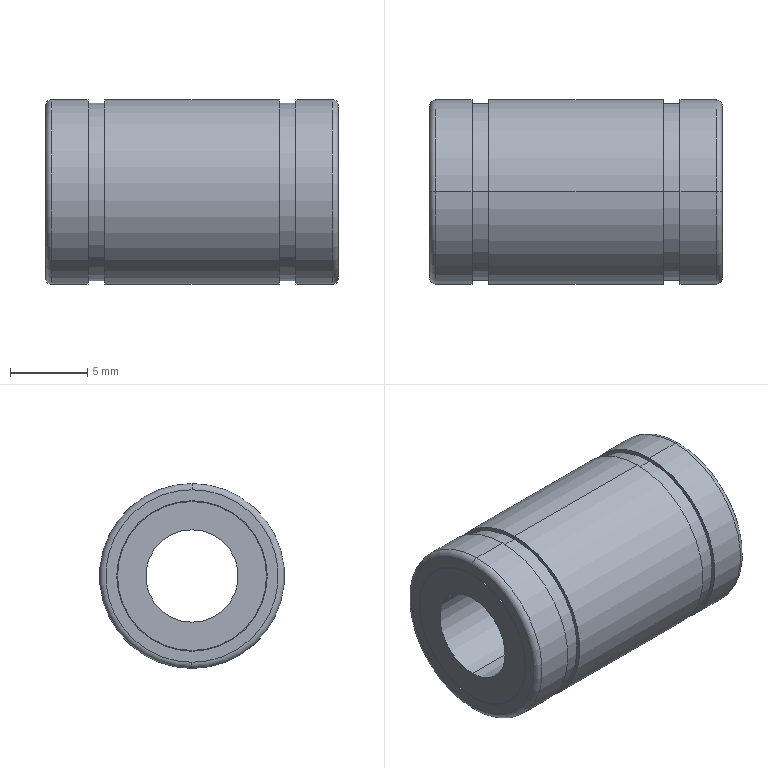Part | STEP file | 11-LMU6-A11_C-LMU6 | 1 solid | 34 faces | box 19 x 12 x 12 mm | volume 1589 mm3 | cylinder 20 | plane 10 | torus 4 | commonest cylinder face diameters 12 x6 9.667 x4 9.767 x4 11.5 x4 6 x2
STEP:
#1=CARTESIAN_POINT('',(9.5,0.,-3.));
#2=VERTEX_POINT('',#1);
#3=CARTESIAN_POINT('',(9.5,0.,3.));
#4=VERTEX_POINT('',#3);
#5=CARTESIAN_POINT('',(9.5,0.,0.));
#6=DIRECTION('',(-1.,0.,0.));
#7=DIRECTION('',(0.,0.,1.));
#8=AXIS2_PLACEMENT_3D('',#5,#6,#7);
#9=CIRCLE('',#8,3.);
#10=EDGE_CURVE('',#2,#4,#9,.T.);
#11=ORIENTED_EDGE('',*,*,#10,.F.);
#12=CARTESIAN_POINT('',(-9.5,0.,-3.));
#13=VERTEX_POINT('',#12);
#14=CARTESIAN_POINT('',(9.5,0.,-3.));
#15=DIRECTION('',(-1.,0.,0.));
#16=VECTOR('',#15,1000.);
#17=LINE('',#14,#16);
#18=EDGE_CURVE('',#2,#13,#17,.T.);
#19=ORIENTED_EDGE('',*,*,#18,.T.);
#20=CARTESIAN_POINT('',(-9.5,0.,3.));
#21=VERTEX_POINT('',#20);
#22=CARTESIAN_POINT('',(-9.5,0.,0.));
#23=DIRECTION('',(-1.,0.,0.));
#24=DIRECTION('',(0.,0.,1.));
#25=AXIS2_PLACEMENT_3D('',#22,#23,#24);
#26=CIRCLE('',#25,3.);
#27=EDGE_CURVE('',#13,#21,#26,.T.);
#28=ORIENTED_EDGE('',*,*,#27,.T.);
#29=CARTESIAN_POINT('',(9.5,0.,3.));
#30=DIRECTION('',(-1.,0.,0.));
#31=VECTOR('',#30,1000.);
#32=LINE('',#29,#31);
#33=EDGE_CURVE('',#4,#21,#32,.T.);
#34=ORIENTED_EDGE('',*,*,#33,.F.);
#35=EDGE_LOOP('',(#11,#19,#28,#34));
#36=FACE_OUTER_BOUND('',#35,.T.);
#37=CARTESIAN_POINT('',(9.5,0.,0.));
#38=DIRECTION('',(-1.,0.,0.));
#39=DIRECTION('',(0.,0.,1.));
#40=AXIS2_PLACEMENT_3D('',#37,#38,#39);
#41=CYLINDRICAL_SURFACE('',#40,3.);
#42=ADVANCED_FACE('',(#36),#41,.F.);
#43=CARTESIAN_POINT('',(9.5,0.,4.833));
#44=VERTEX_POINT('',#43);
#45=CARTESIAN_POINT('',(9.5,0.,-4.833));
#46=VERTEX_POINT('',#45);
#47=CARTESIAN_POINT('',(9.5,0.,0.));
#48=DIRECTION('',(-1.,0.,0.));
#49=DIRECTION('',(0.,0.,1.));
#50=AXIS2_PLACEMENT_3D('',#47,#48,#49);
#51=CIRCLE('',#50,4.833);
#52=EDGE_CURVE('',#44,#46,#51,.T.);
#53=ORIENTED_EDGE('',*,*,#52,.T.);
#54=CARTESIAN_POINT('',(9.45,0.,-4.833));
#55=VERTEX_POINT('',#54);
#56=CARTESIAN_POINT('',(9.5,0.,-4.833));
#57=DIRECTION('',(-1.,0.,0.));
#58=VECTOR('',#57,1000.);
#59=LINE('',#56,#58);
#60=EDGE_CURVE('',#46,#55,#59,.T.);
#61=ORIENTED_EDGE('',*,*,#60,.T.);
#62=CARTESIAN_POINT('',(9.45,0.,4.833));
#63=VERTEX_POINT('',#62);
#64=CARTESIAN_POINT('',(9.45,0.,0.));
#65=DIRECTION('',(1.,0.,0.));
#66=DIRECTION('',(0.,0.,1.));
#67=AXIS2_PLACEMENT_3D('',#64,#65,#66);
#68=CIRCLE('',#67,4.833);
#69=EDGE_CURVE('',#55,#63,#68,.T.);
#70=ORIENTED_EDGE('',*,*,#69,.T.);
#71=CARTESIAN_POINT('',(9.5,0.,4.833));
#72=DIRECTION('',(-1.,0.,0.));
#73=VECTOR('',#72,1000.);
#74=LINE('',#71,#73);
#75=EDGE_CURVE('',#44,#63,#74,.T.);
#76=ORIENTED_EDGE('',*,*,#75,.F.);
#77=EDGE_LOOP('',(#53,#61,#70,#76));
#78=FACE_OUTER_BOUND('',#77,.T.);
#79=CARTESIAN_POINT('',(9.5,0.,0.));
#80=DIRECTION('',(-1.,0.,0.));
#81=DIRECTION('',(0.,0.,1.));
#82=AXIS2_PLACEMENT_3D('',#79,#80,#81);
#83=CYLINDRICAL_SURFACE('',#82,4.833);
#84=ADVANCED_FACE('',(#78),#83,.T.);
#85=CARTESIAN_POINT('',(-9.45,0.,4.833));
#86=VERTEX_POINT('',#85);
#87=CARTESIAN_POINT('',(-9.45,0.,-4.833));
#88=VERTEX_POINT('',#87);
#89=CARTESIAN_POINT('',(-9.45,0.,0.));
#90=DIRECTION('',(-1.,0.,0.));
#91=DIRECTION('',(0.,0.,1.));
#92=AXIS2_PLACEMENT_3D('',#89,#90,#91);
#93=CIRCLE('',#92,4.833);
#94=EDGE_CURVE('',#86,#88,#93,.T.);
#95=ORIENTED_EDGE('',*,*,#94,.T.);
#96=CARTESIAN_POINT('',(-9.5,0.,-4.833));
#97=VERTEX_POINT('',#96);
#98=CARTESIAN_POINT('',(9.5,0.,-4.833));
#99=DIRECTION('',(-1.,0.,0.));
#100=VECTOR('',#99,1000.);
#101=LINE('',#98,#100);
#102=EDGE_CURVE('',#88,#97,#101,.T.);
#103=ORIENTED_EDGE('',*,*,#102,.T.);
#104=CARTESIAN_POINT('',(-9.5,0.,4.833));
#105=VERTEX_POINT('',#104);
#106=CARTESIAN_POINT('',(-9.5,0.,0.));
#107=DIRECTION('',(-1.,0.,0.));
#108=DIRECTION('',(0.,0.,1.));
#109=AXIS2_PLACEMENT_3D('',#106,#107,#108);
#110=CIRCLE('',#109,4.833);
#111=EDGE_CURVE('',#105,#97,#110,.T.);
#112=ORIENTED_EDGE('',*,*,#111,.F.);
#113=CARTESIAN_POINT('',(9.5,0.,4.833));
#114=DIRECTION('',(-1.,0.,0.));
#115=VECTOR('',#114,1000.);
#116=LINE('',#113,#115);
#117=EDGE_CURVE('',#86,#105,#116,.T.);
#118=ORIENTED_EDGE('',*,*,#117,.F.);
#119=EDGE_LOOP('',(#95,#103,#112,#118));
#120=FACE_OUTER_BOUND('',#119,.T.);
#121=CARTESIAN_POINT('',(9.5,0.,0.));
#122=DIRECTION('',(-1.,0.,0.));
#123=DIRECTION('',(0.,0.,1.));
#124=AXIS2_PLACEMENT_3D('',#121,#122,#123);
#125=CYLINDRICAL_SURFACE('',#124,4.833);
#126=ADVANCED_FACE('',(#120),#125,.T.);
#127=CARTESIAN_POINT('',(-9.1,0.,6.));
#128=VERTEX_POINT('',#127);
#129=CARTESIAN_POINT('',(-9.1,0.,-6.));
#130=VERTEX_POINT('',#129);
#131=CARTESIAN_POINT('',(-9.1,0.,0.));
#132=DIRECTION('',(-1.,0.,0.));
#133=DIRECTION('',(0.,0.,1.));
#134=AXIS2_PLACEMENT_3D('',#131,#132,#133);
#135=CIRCLE('',#134,6.);
#136=EDGE_CURVE('',#128,#130,#135,.T.);
#137=ORIENTED_EDGE('',*,*,#136,.T.);
#138=CARTESIAN_POINT('',(-9.5,0.,-5.6));
#139=VERTEX_POINT('',#138);
#140=CARTESIAN_POINT('',(-9.1,0.,-5.6));
#141=DIRECTION('',(0.,1.,0.));
#142=DIRECTION('',(0.,0.,1.));
#143=AXIS2_PLACEMENT_3D('',#140,#141,#142);
#144=CIRCLE('',#143,0.4);
#145=EDGE_CURVE('',#130,#139,#144,.T.);
#146=ORIENTED_EDGE('',*,*,#145,.T.);
#147=CARTESIAN_POINT('',(-9.5,0.,5.6));
#148=VERTEX_POINT('',#147);
#149=CARTESIAN_POINT('',(-9.5,0.,0.));
#150=DIRECTION('',(-1.,0.,0.));
#151=DIRECTION('',(0.,0.,1.));
#152=AXIS2_PLACEMENT_3D('',#149,#150,#151);
#153=CIRCLE('',#152,5.6);
#154=EDGE_CURVE('',#148,#139,#153,.T.);
#155=ORIENTED_EDGE('',*,*,#154,.F.);
#156=CARTESIAN_POINT('',(-9.1,0.,5.6));
#157=DIRECTION('',(0.,-1.,0.));
#158=DIRECTION('',(0.,0.,-1.));
#159=AXIS2_PLACEMENT_3D('',#156,#157,#158);
#160=CIRCLE('',#159,0.4);
#161=EDGE_CURVE('',#128,#148,#160,.T.);
#162=ORIENTED_EDGE('',*,*,#161,.F.);
#163=EDGE_LOOP('',(#137,#146,#155,#162));
#164=FACE_OUTER_BOUND('',#163,.T.);
#165=CARTESIAN_POINT('',(-9.1,0.,0.));
#166=DIRECTION('',(-1.,0.,0.));
#167=DIRECTION('',(0.,0.,1.));
#168=AXIS2_PLACEMENT_3D('',#165,#166,#167);
#169=TOROIDAL_SURFACE('',#168,5.6,0.4);
#170=ADVANCED_FACE('',(#164),#169,.T.);
#171=CARTESIAN_POINT('',(-6.75,0.,6.));
#172=VERTEX_POINT('',#171);
#173=CARTESIAN_POINT('',(-6.75,0.,-6.));
#174=VERTEX_POINT('',#173);
#175=CARTESIAN_POINT('',(-6.75,0.,0.));
#176=DIRECTION('',(-1.,0.,0.));
#177=DIRECTION('',(0.,0.,1.));
#178=AXIS2_PLACEMENT_3D('',#175,#176,#177);
#179=CIRCLE('',#178,6.);
#180=EDGE_CURVE('',#172,#174,#179,.T.);
#181=ORIENTED_EDGE('',*,*,#180,.T.);
#182=CARTESIAN_POINT('',(9.5,0.,-6.));
#183=DIRECTION('',(-1.,0.,0.));
#184=VECTOR('',#183,1000.);
#185=LINE('',#182,#184);
#186=EDGE_CURVE('',#174,#130,#185,.T.);
#187=ORIENTED_EDGE('',*,*,#186,.T.);
#188=ORIENTED_EDGE('',*,*,#136,.F.);
#189=CARTESIAN_POINT('',(9.5,0.,6.));
#190=DIRECTION('',(-1.,0.,0.));
#191=VECTOR('',#190,1000.);
#192=LINE('',#189,#191);
#193=EDGE_CURVE('',#172,#128,#192,.T.);
#194=ORIENTED_EDGE('',*,*,#193,.F.);
#195=EDGE_LOOP('',(#181,#187,#188,#194));
#196=FACE_OUTER_BOUND('',#195,.T.);
#197=CARTESIAN_POINT('',(9.5,0.,0.));
#198=DIRECTION('',(-1.,0.,0.));
#199=DIRECTION('',(0.,0.,1.));
#200=AXIS2_PLACEMENT_3D('',#197,#198,#199);
#201=CYLINDRICAL_SURFACE('',#200,6.);
#202=ADVANCED_FACE('',(#196),#201,.T.);
#203=CARTESIAN_POINT('',(-5.65,0.,5.75));
#204=VERTEX_POINT('',#203);
#205=CARTESIAN_POINT('',(-5.65,0.,-5.75));
#206=VERTEX_POINT('',#205);
#207=CARTESIAN_POINT('',(-5.65,0.,0.));
#208=DIRECTION('',(-1.,0.,0.));
#209=DIRECTION('',(0.,0.,1.));
#210=AXIS2_PLACEMENT_3D('',#207,#208,#209);
#211=CIRCLE('',#210,5.75);
#212=EDGE_CURVE('',#204,#206,#211,.T.);
#213=ORIENTED_EDGE('',*,*,#212,.T.);
#214=CARTESIAN_POINT('',(-6.75,0.,-5.75));
#215=VERTEX_POINT('',#214);
#216=CARTESIAN_POINT('',(9.5,0.,-5.75));
#217=DIRECTION('',(-1.,0.,0.));
#218=VECTOR('',#217,1000.);
#219=LINE('',#216,#218);
#220=EDGE_CURVE('',#206,#215,#219,.T.);
#221=ORIENTED_EDGE('',*,*,#220,.T.);
#222=CARTESIAN_POINT('',(-6.75,0.,5.75));
#223=VERTEX_POINT('',#222);
#224=CARTESIAN_POINT('',(-6.75,0.,0.));
#225=DIRECTION('',(-1.,0.,0.));
#226=DIRECTION('',(0.,0.,1.));
#227=AXIS2_PLACEMENT_3D('',#224,#225,#226);
#228=CIRCLE('',#227,5.75);
#229=EDGE_CURVE('',#223,#215,#228,.T.);
#230=ORIENTED_EDGE('',*,*,#229,.F.);
#231=CARTESIAN_POINT('',(9.5,0.,5.75));
#232=DIRECTION('',(-1.,0.,0.));
#233=VECTOR('',#232,1000.);
#234=LINE('',#231,#233);
#235=EDGE_CURVE('',#204,#223,#234,.T.);
#236=ORIENTED_EDGE('',*,*,#235,.F.);
#237=EDGE_LOOP('',(#213,#221,#230,#236));
#238=FACE_OUTER_BOUND('',#237,.T.);
#239=CARTESIAN_POINT('',(9.5,0.,0.));
#240=DIRECTION('',(-1.,0.,0.));
#241=DIRECTION('',(0.,0.,1.));
#242=AXIS2_PLACEMENT_3D('',#239,#240,#241);
#243=CYLINDRICAL_SURFACE('',#242,5.75);
#244=ADVANCED_FACE('',(#238),#243,.T.);
#245=CARTESIAN_POINT('',(5.65,0.,6.));
#246=VERTEX_POINT('',#245);
#247=CARTESIAN_POINT('',(5.65,0.,-6.));
#248=VERTEX_POINT('',#247);
#249=CARTESIAN_POINT('',(5.65,0.,0.));
#250=DIRECTION('',(-1.,0.,0.));
#251=DIRECTION('',(0.,0.,1.));
#252=AXIS2_PLACEMENT_3D('',#249,#250,#251);
#253=CIRCLE('',#252,6.);
#254=EDGE_CURVE('',#246,#248,#253,.T.);
#255=ORIENTED_EDGE('',*,*,#254,.T.);
#256=CARTESIAN_POINT('',(-5.65,0.,-6.));
#257=VERTEX_POINT('',#256);
#258=CARTESIAN_POINT('',(9.5,0.,-6.));
#259=DIRECTION('',(-1.,0.,0.));
#260=VECTOR('',#259,1000.);
#261=LINE('',#258,#260);
#262=EDGE_CURVE('',#248,#257,#261,.T.);
#263=ORIENTED_EDGE('',*,*,#262,.T.);
#264=CARTESIAN_POINT('',(-5.65,0.,6.));
#265=VERTEX_POINT('',#264);
#266=CARTESIAN_POINT('',(-5.65,0.,0.));
#267=DIRECTION('',(-1.,0.,0.));
#268=DIRECTION('',(0.,0.,1.));
#269=AXIS2_PLACEMENT_3D('',#266,#267,#268);
#270=CIRCLE('',#269,6.);
#271=EDGE_CURVE('',#265,#257,#270,.T.);
#272=ORIENTED_EDGE('',*,*,#271,.F.);
#273=CARTESIAN_POINT('',(9.5,0.,6.));
#274=DIRECTION('',(-1.,0.,0.));
#275=VECTOR('',#274,1000.);
#276=LINE('',#273,#275);
#277=EDGE_CURVE('',#246,#265,#276,.T.);
#278=ORIENTED_EDGE('',*,*,#277,.F.);
#279=EDGE_LOOP('',(#255,#263,#272,#278));
#280=FACE_OUTER_BOUND('',#279,.T.);
#281=CARTESIAN_POINT('',(9.5,0.,0.));
#282=DIRECTION('',(-1.,0.,0.));
#283=DIRECTION('',(0.,0.,1.));
#284=AXIS2_PLACEMENT_3D('',#281,#282,#283);
#285=CYLINDRICAL_SURFACE('',#284,6.);
#286=ADVANCED_FACE('',(#280),#285,.T.);
#287=CARTESIAN_POINT('',(6.75,0.,5.75));
#288=VERTEX_POINT('',#287);
#289=CARTESIAN_POINT('',(6.75,0.,-5.75));
#290=VERTEX_POINT('',#289);
#291=CARTESIAN_POINT('',(6.75,0.,0.));
#292=DIRECTION('',(-1.,0.,0.));
#293=DIRECTION('',(0.,0.,1.));
#294=AXIS2_PLACEMENT_3D('',#291,#292,#293);
#295=CIRCLE('',#294,5.75);
#296=EDGE_CURVE('',#288,#290,#295,.T.);
#297=ORIENTED_EDGE('',*,*,#296,.T.);
#298=CARTESIAN_POINT('',(5.65,0.,-5.75));
#299=VERTEX_POINT('',#298);
#300=CARTESIAN_POINT('',(9.5,0.,-5.75));
#301=DIRECTION('',(-1.,0.,0.));
#302=VECTOR('',#301,1000.);
#303=LINE('',#300,#302);
#304=EDGE_CURVE('',#290,#299,#303,.T.);
#305=ORIENTED_EDGE('',*,*,#304,.T.);
#306=CARTESIAN_POINT('',(5.65,0.,5.75));
#307=VERTEX_POINT('',#306);
#308=CARTESIAN_POINT('',(5.65,0.,0.));
#309=DIRECTION('',(-1.,0.,0.));
#310=DIRECTION('',(0.,0.,1.));
#311=AXIS2_PLACEMENT_3D('',#308,#309,#310);
#312=CIRCLE('',#311,5.75);
#313=EDGE_CURVE('',#307,#299,#312,.T.);
#314=ORIENTED_EDGE('',*,*,#313,.F.);
#315=CARTESIAN_POINT('',(9.5,0.,5.75));
#316=DIRECTION('',(-1.,0.,0.));
#317=VECTOR('',#316,1000.);
#318=LINE('',#315,#317);
#319=EDGE_CURVE('',#288,#307,#318,.T.);
#320=ORIENTED_EDGE('',*,*,#319,.F.);
#321=EDGE_LOOP('',(#297,#305,#314,#320));
#322=FACE_OUTER_BOUND('',#321,.T.);
#323=CARTESIAN_POINT('',(9.5,0.,0.));
#324=DIRECTION('',(-1.,0.,0.));
#325=DIRECTION('',(0.,0.,1.));
#326=AXIS2_PLACEMENT_3D('',#323,#324,#325);
#327=CYLINDRICAL_SURFACE('',#326,5.75);
#328=ADVANCED_FACE('',(#322),#327,.T.);
#329=CARTESIAN_POINT('',(9.1,0.,6.));
#330=VERTEX_POINT('',#329);
#331=CARTESIAN_POINT('',(9.1,0.,-6.));
#332=VERTEX_POINT('',#331);
#333=CARTESIAN_POINT('',(9.1,0.,0.));
#334=DIRECTION('',(-1.,0.,0.));
#335=DIRECTION('',(0.,0.,1.));
#336=AXIS2_PLACEMENT_3D('',#333,#334,#335);
#337=CIRCLE('',#336,6.);
#338=EDGE_CURVE('',#330,#332,#337,.T.);
#339=ORIENTED_EDGE('',*,*,#338,.T.);
#340=CARTESIAN_POINT('',(6.75,0.,-6.));
#341=VERTEX_POINT('',#340);
#342=CARTESIAN_POINT('',(9.5,0.,-6.));
#343=DIRECTION('',(-1.,0.,0.));
#344=VECTOR('',#343,1000.);
#345=LINE('',#342,#344);
#346=EDGE_CURVE('',#332,#341,#345,.T.);
#347=ORIENTED_EDGE('',*,*,#346,.T.);
#348=CARTESIAN_POINT('',(6.75,0.,6.));
#349=VERTEX_POINT('',#348);
#350=CARTESIAN_POINT('',(6.75,0.,0.));
#351=DIRECTION('',(-1.,0.,0.));
#352=DIRECTION('',(0.,0.,1.));
#353=AXIS2_PLACEMENT_3D('',#350,#351,#352);
#354=CIRCLE('',#353,6.);
#355=EDGE_CURVE('',#349,#341,#354,.T.);
#356=ORIENTED_EDGE('',*,*,#355,.F.);
#357=CARTESIAN_POINT('',(9.5,0.,6.));
#358=DIRECTION('',(-1.,0.,0.));
#359=VECTOR('',#358,1000.);
#360=LINE('',#357,#359);
#361=EDGE_CURVE('',#330,#349,#360,.T.);
#362=ORIENTED_EDGE('',*,*,#361,.F.);
#363=EDGE_LOOP('',(#339,#347,#356,#362));
#364=FACE_OUTER_BOUND('',#363,.T.);
#365=CARTESIAN_POINT('',(9.5,0.,0.));
#366=DIRECTION('',(-1.,0.,0.));
#367=DIRECTION('',(0.,0.,1.));
#368=AXIS2_PLACEMENT_3D('',#365,#366,#367);
#369=CYLINDRICAL_SURFACE('',#368,6.);
#370=ADVANCED_FACE('',(#364),#369,.T.);
#371=CARTESIAN_POINT('',(9.5,0.,5.6));
#372=VERTEX_POINT('',#371);
#373=CARTESIAN_POINT('',(9.5,0.,-5.6));
#374=VERTEX_POINT('',#373);
#375=CARTESIAN_POINT('',(9.5,0.,0.));
#376=DIRECTION('',(-1.,0.,0.));
#377=DIRECTION('',(0.,0.,1.));
#378=AXIS2_PLACEMENT_3D('',#375,#376,#377);
#379=CIRCLE('',#378,5.6);
#380=EDGE_CURVE('',#372,#374,#379,.T.);
#381=ORIENTED_EDGE('',*,*,#380,.T.);
#382=CARTESIAN_POINT('',(9.1,0.,-5.6));
#383=DIRECTION('',(0.,1.,0.));
#384=DIRECTION('',(0.,0.,1.));
#385=AXIS2_PLACEMENT_3D('',#382,#383,#384);
#386=CIRCLE('',#385,0.4);
#387=EDGE_CURVE('',#374,#332,#386,.T.);
#388=ORIENTED_EDGE('',*,*,#387,.T.);
#389=ORIENTED_EDGE('',*,*,#338,.F.);
#390=CARTESIAN_POINT('',(9.1,0.,5.6));
#391=DIRECTION('',(0.,-1.,0.));
#392=DIRECTION('',(0.,0.,-1.));
#393=AXIS2_PLACEMENT_3D('',#390,#391,#392);
#394=CIRCLE('',#393,0.4);
#395=EDGE_CURVE('',#372,#330,#394,.T.);
#396=ORIENTED_EDGE('',*,*,#395,.F.);
#397=EDGE_LOOP('',(#381,#388,#389,#396));
#398=FACE_OUTER_BOUND('',#397,.T.);
#399=CARTESIAN_POINT('',(9.1,0.,0.));
#400=DIRECTION('',(-1.,0.,0.));
#401=DIRECTION('',(0.,0.,1.));
#402=AXIS2_PLACEMENT_3D('',#399,#400,#401);
#403=TOROIDAL_SURFACE('',#402,5.6,0.4);
#404=ADVANCED_FACE('',(#398),#403,.T.);
#405=CARTESIAN_POINT('',(9.5,0.,-4.883));
#406=VERTEX_POINT('',#405);
#407=CARTESIAN_POINT('',(9.5,0.,4.883));
#408=VERTEX_POINT('',#407);
#409=CARTESIAN_POINT('',(9.5,0.,0.));
#410=DIRECTION('',(-1.,0.,0.));
#411=DIRECTION('',(0.,0.,1.));
#412=AXIS2_PLACEMENT_3D('',#409,#410,#411);
#413=CIRCLE('',#412,4.883);
#414=EDGE_CURVE('',#406,#408,#413,.T.);
#415=ORIENTED_EDGE('',*,*,#414,.F.);
#416=CARTESIAN_POINT('',(9.45,0.,-4.883));
#417=VERTEX_POINT('',#416);
#418=CARTESIAN_POINT('',(9.5,0.,-4.883));
#419=DIRECTION('',(-1.,0.,0.));
#420=VECTOR('',#419,1000.);
#421=LINE('',#418,#420);
#422=EDGE_CURVE('',#406,#417,#421,.T.);
#423=ORIENTED_EDGE('',*,*,#422,.T.);
#424=CARTESIAN_POINT('',(9.45,0.,4.883));
#425=VERTEX_POINT('',#424);
#426=CARTESIAN_POINT('',(9.45,0.,0.));
#427=DIRECTION('',(-1.,0.,0.));
#428=DIRECTION('',(0.,0.,1.));
#429=AXIS2_PLACEMENT_3D('',#426,#427,#428);
#430=CIRCLE('',#429,4.883);
#431=EDGE_CURVE('',#417,#425,#430,.T.);
#432=ORIENTED_EDGE('',*,*,#431,.T.);
#433=CARTESIAN_POINT('',(9.5,0.,4.883));
#434=DIRECTION('',(-1.,0.,0.));
#435=VECTOR('',#434,1000.);
#436=LINE('',#433,#435);
#437=EDGE_CURVE('',#408,#425,#436,.T.);
#438=ORIENTED_EDGE('',*,*,#437,.F.);
#439=EDGE_LOOP('',(#415,#423,#432,#438));
#440=FACE_OUTER_BOUND('',#439,.T.);
#441=CARTESIAN_POINT('',(9.5,0.,0.));
#442=DIRECTION('',(-1.,0.,0.));
#443=DIRECTION('',(0.,0.,1.));
#444=AXIS2_PLACEMENT_3D('',#441,#442,#443);
#445=CYLINDRICAL_SURFACE('',#444,4.883);
#446=ADVANCED_FACE('',(#440),#445,.F.);
#447=CARTESIAN_POINT('',(-9.45,0.,-4.883));
#448=VERTEX_POINT('',#447);
#449=CARTESIAN_POINT('',(-9.45,0.,4.883));
#450=VERTEX_POINT('',#449);
#451=CARTESIAN_POINT('',(-9.45,0.,0.));
#452=DIRECTION('',(-1.,0.,0.));
#453=DIRECTION('',(0.,0.,1.));
#454=AXIS2_PLACEMENT_3D('',#451,#452,#453);
#455=CIRCLE('',#454,4.883);
#456=EDGE_CURVE('',#448,#450,#455,.T.);
#457=ORIENTED_EDGE('',*,*,#456,.F.);
#458=CARTESIAN_POINT('',(-9.5,0.,-4.883));
#459=VERTEX_POINT('',#458);
#460=CARTESIAN_POINT('',(9.5,0.,-4.883));
#461=DIRECTION('',(-1.,0.,0.));
#462=VECTOR('',#461,1000.);
#463=LINE('',#460,#462);
#464=EDGE_CURVE('',#448,#459,#463,.T.);
#465=ORIENTED_EDGE('',*,*,#464,.T.);
#466=CARTESIAN_POINT('',(-9.5,0.,4.883));
#467=VERTEX_POINT('',#466);
#468=CARTESIAN_POINT('',(-9.5,0.,0.));
#469=DIRECTION('',(-1.,0.,0.));
#470=DIRECTION('',(0.,0.,1.));
#471=AXIS2_PLACEMENT_3D('',#468,#469,#470);
#472=CIRCLE('',#471,4.883);
#473=EDGE_CURVE('',#459,#467,#472,.T.);
#474=ORIENTED_EDGE('',*,*,#473,.T.);
#475=CARTESIAN_POINT('',(9.5,0.,4.883));
#476=DIRECTION('',(-1.,0.,0.));
#477=VECTOR('',#476,1000.);
#478=LINE('',#475,#477);
#479=EDGE_CURVE('',#450,#467,#478,.T.);
#480=ORIENTED_EDGE('',*,*,#479,.F.);
#481=EDGE_LOOP('',(#457,#465,#474,#480));
#482=FACE_OUTER_BOUND('',#481,.T.);
#483=CARTESIAN_POINT('',(9.5,0.,0.));
#484=DIRECTION('',(-1.,0.,0.));
#485=DIRECTION('',(0.,0.,1.));
#486=AXIS2_PLACEMENT_3D('',#483,#484,#485);
#487=CYLINDRICAL_SURFACE('',#486,4.883);
#488=ADVANCED_FACE('',(#482),#487,.F.);
#489=CARTESIAN_POINT('',(-9.5,0.,0.));
#490=DIRECTION('',(-1.,0.,0.));
#491=DIRECTION('',(0.,0.,1.));
#492=AXIS2_PLACEMENT_3D('',#489,#490,#491);
#493=CIRCLE('',#492,4.883);
#494=EDGE_CURVE('',#467,#459,#493,.T.);
#495=ORIENTED_EDGE('',*,*,#494,.F.);
#496=ORIENTED_EDGE('',*,*,#473,.F.);
#497=EDGE_LOOP('',(#495,#496));
#498=FACE_BOUND('',#497,.T.);
#499=ORIENTED_EDGE('',*,*,#154,.T.);
#500=CARTESIAN_POINT('',(-9.5,0.,0.));
#501=DIRECTION('',(-1.,0.,0.));
#502=DIRECTION('',(0.,0.,1.));
#503=AXIS2_PLACEMENT_3D('',#500,#501,#502);
#504=CIRCLE('',#503,5.6);
#505=EDGE_CURVE('',#139,#148,#504,.T.);
#506=ORIENTED_EDGE('',*,*,#505,.T.);
#507=EDGE_LOOP('',(#499,#506));
#508=FACE_OUTER_BOUND('',#507,.T.);
#509=CARTESIAN_POINT('',(-9.5,5.6,0.));
#510=DIRECTION('',(1.,0.,0.));
#511=DIRECTION('',(0.,0.,-1.));
#512=AXIS2_PLACEMENT_3D('',#509,#510,#511);
#513=PLANE('',#512);
#514=ADVANCED_FACE('',(#498,#508),#513,.F.);
#515=ORIENTED_EDGE('',*,*,#464,.F.);
#516=CARTESIAN_POINT('',(-9.45,0.,0.));
#517=DIRECTION('',(-1.,0.,0.));
#518=DIRECTION('',(0.,0.,1.));
#519=AXIS2_PLACEMENT_3D('',#516,#517,#518);
#520=CIRCLE('',#519,4.883);
#521=EDGE_CURVE('',#450,#448,#520,.T.);
#522=ORIENTED_EDGE('',*,*,#521,.F.);
#523=ORIENTED_EDGE('',*,*,#479,.T.);
#524=ORIENTED_EDGE('',*,*,#494,.T.);
#525=EDGE_LOOP('',(#515,#522,#523,#524));
#526=FACE_OUTER_BOUND('',#525,.T.);
#527=CARTESIAN_POINT('',(9.5,0.,0.));
#528=DIRECTION('',(-1.,0.,0.));
#529=DIRECTION('',(0.,0.,1.));
#530=AXIS2_PLACEMENT_3D('',#527,#528,#529);
#531=CYLINDRICAL_SURFACE('',#530,4.883);
#532=ADVANCED_FACE('',(#526),#531,.F.);
#533=ORIENTED_EDGE('',*,*,#94,.F.);
#534=CARTESIAN_POINT('',(-9.45,0.,0.));
#535=DIRECTION('',(-1.,0.,0.));
#536=DIRECTION('',(0.,0.,1.));
#537=AXIS2_PLACEMENT_3D('',#534,#535,#536);
#538=CIRCLE('',#537,4.833);
#539=EDGE_CURVE('',#88,#86,#538,.T.);
#540=ORIENTED_EDGE('',*,*,#539,.F.);
#541=EDGE_LOOP('',(#533,#540));
#542=FACE_BOUND('',#541,.T.);
#543=ORIENTED_EDGE('',*,*,#521,.T.);
#544=ORIENTED_EDGE('',*,*,#456,.T.);
#545=EDGE_LOOP('',(#543,#544));
#546=FACE_OUTER_BOUND('',#545,.T.);
#547=CARTESIAN_POINT('',(-9.45,4.883,0.));
#548=DIRECTION('',(1.,0.,0.));
#549=DIRECTION('',(0.,0.,-1.));
#550=AXIS2_PLACEMENT_3D('',#547,#548,#549);
#551=PLANE('',#550);
#552=ADVANCED_FACE('',(#542,#546),#551,.F.);
#553=CARTESIAN_POINT('',(9.45,0.,0.));
#554=DIRECTION('',(-1.,0.,0.));
#555=DIRECTION('',(0.,0.,1.));
#556=AXIS2_PLACEMENT_3D('',#553,#554,#555);
#557=CIRCLE('',#556,4.883);
#558=EDGE_CURVE('',#425,#417,#557,.T.);
#559=ORIENTED_EDGE('',*,*,#558,.F.);
#560=ORIENTED_EDGE('',*,*,#431,.F.);
#561=EDGE_LOOP('',(#559,#560));
#562=FACE_OUTER_BOUND('',#561,.T.);
#563=CARTESIAN_POINT('',(9.45,0.,0.));
#564=DIRECTION('',(1.,0.,0.));
#565=DIRECTION('',(0.,0.,1.));
#566=AXIS2_PLACEMENT_3D('',#563,#564,#565);
#567=CIRCLE('',#566,4.833);
#568=EDGE_CURVE('',#63,#55,#567,.T.);
#569=ORIENTED_EDGE('',*,*,#568,.F.);
#570=ORIENTED_EDGE('',*,*,#69,.F.);
#571=EDGE_LOOP('',(#569,#570));
#572=FACE_BOUND('',#571,.T.);
#573=CARTESIAN_POINT('',(9.45,4.833,0.));
#574=DIRECTION('',(-1.,0.,0.));
#575=DIRECTION('',(0.,0.,1.));
#576=AXIS2_PLACEMENT_3D('',#573,#574,#575);
#577=PLANE('',#576);
#578=ADVANCED_FACE('',(#562,#572),#577,.F.);
#579=ORIENTED_EDGE('',*,*,#422,.F.);
#580=CARTESIAN_POINT('',(9.5,0.,0.));
#581=DIRECTION('',(-1.,0.,0.));
#582=DIRECTION('',(0.,0.,1.));
#583=AXIS2_PLACEMENT_3D('',#580,#581,#582);
#584=CIRCLE('',#583,4.883);
#585=EDGE_CURVE('',#408,#406,#584,.T.);
#586=ORIENTED_EDGE('',*,*,#585,.F.);
#587=ORIENTED_EDGE('',*,*,#437,.T.);
#588=ORIENTED_EDGE('',*,*,#558,.T.);
#589=EDGE_LOOP('',(#579,#586,#587,#588));
#590=FACE_OUTER_BOUND('',#589,.T.);
#591=CARTESIAN_POINT('',(9.5,0.,0.));
#592=DIRECTION('',(-1.,0.,0.));
#593=DIRECTION('',(0.,0.,1.));
#594=AXIS2_PLACEMENT_3D('',#591,#592,#593);
#595=CYLINDRICAL_SURFACE('',#594,4.883);
#596=ADVANCED_FACE('',(#590),#595,.F.);
#597=ORIENTED_EDGE('',*,*,#380,.F.);
#598=CARTESIAN_POINT('',(9.5,0.,0.));
#599=DIRECTION('',(-1.,0.,0.));
#600=DIRECTION('',(0.,0.,1.));
#601=AXIS2_PLACEMENT_3D('',#598,#599,#600);
#602=CIRCLE('',#601,5.6);
#603=EDGE_CURVE('',#374,#372,#602,.T.);
#604=ORIENTED_EDGE('',*,*,#603,.F.);
#605=EDGE_LOOP('',(#597,#604));
#606=FACE_OUTER_BOUND('',#605,.T.);
#607=ORIENTED_EDGE('',*,*,#585,.T.);
#608=ORIENTED_EDGE('',*,*,#414,.T.);
#609=EDGE_LOOP('',(#607,#608));
#610=FACE_BOUND('',#609,.T.);
#611=CARTESIAN_POINT('',(9.5,4.883,0.));
#612=DIRECTION('',(-1.,0.,0.));
#613=DIRECTION('',(0.,0.,1.));
#614=AXIS2_PLACEMENT_3D('',#611,#612,#613);
#615=PLANE('',#614);
#616=ADVANCED_FACE('',(#606,#610),#615,.F.);
#617=ORIENTED_EDGE('',*,*,#387,.F.);
#618=ORIENTED_EDGE('',*,*,#603,.T.);
#619=ORIENTED_EDGE('',*,*,#395,.T.);
#620=CARTESIAN_POINT('',(9.1,0.,0.));
#621=DIRECTION('',(-1.,0.,0.));
#622=DIRECTION('',(0.,0.,1.));
#623=AXIS2_PLACEMENT_3D('',#620,#621,#622);
#624=CIRCLE('',#623,6.);
#625=EDGE_CURVE('',#332,#330,#624,.T.);
#626=ORIENTED_EDGE('',*,*,#625,.F.);
#627=EDGE_LOOP('',(#617,#618,#619,#626));
#628=FACE_OUTER_BOUND('',#627,.T.);
#629=CARTESIAN_POINT('',(9.1,0.,0.));
#630=DIRECTION('',(-1.,0.,0.));
#631=DIRECTION('',(0.,0.,1.));
#632=AXIS2_PLACEMENT_3D('',#629,#630,#631);
#633=TOROIDAL_SURFACE('',#632,5.6,0.4);
#634=ADVANCED_FACE('',(#628),#633,.T.);
#635=ORIENTED_EDGE('',*,*,#346,.F.);
#636=ORIENTED_EDGE('',*,*,#625,.T.);
#637=ORIENTED_EDGE('',*,*,#361,.T.);
#638=CARTESIAN_POINT('',(6.75,0.,0.));
#639=DIRECTION('',(-1.,0.,0.));
#640=DIRECTION('',(0.,0.,1.));
#641=AXIS2_PLACEMENT_3D('',#638,#639,#640);
#642=CIRCLE('',#641,6.);
#643=EDGE_CURVE('',#341,#349,#642,.T.);
#644=ORIENTED_EDGE('',*,*,#643,.F.);
#645=EDGE_LOOP('',(#635,#636,#637,#644));
#646=FACE_OUTER_BOUND('',#645,.T.);
#647=CARTESIAN_POINT('',(9.5,0.,0.));
#648=DIRECTION('',(-1.,0.,0.));
#649=DIRECTION('',(0.,0.,1.));
#650=AXIS2_PLACEMENT_3D('',#647,#648,#649);
#651=CYLINDRICAL_SURFACE('',#650,6.);
#652=ADVANCED_FACE('',(#646),#651,.T.);
#653=ORIENTED_EDGE('',*,*,#296,.F.);
#654=CARTESIAN_POINT('',(6.75,0.,0.));
#655=DIRECTION('',(-1.,0.,0.));
#656=DIRECTION('',(0.,0.,1.));
#657=AXIS2_PLACEMENT_3D('',#654,#655,#656);
#658=CIRCLE('',#657,5.75);
#659=EDGE_CURVE('',#290,#288,#658,.T.);
#660=ORIENTED_EDGE('',*,*,#659,.F.);
#661=EDGE_LOOP('',(#653,#660));
#662=FACE_BOUND('',#661,.T.);
#663=ORIENTED_EDGE('',*,*,#355,.T.);
#664=ORIENTED_EDGE('',*,*,#643,.T.);
#665=EDGE_LOOP('',(#663,#664));
#666=FACE_OUTER_BOUND('',#665,.T.);
#667=CARTESIAN_POINT('',(6.75,6.,0.));
#668=DIRECTION('',(1.,0.,0.));
#669=DIRECTION('',(0.,0.,-1.));
#670=AXIS2_PLACEMENT_3D('',#667,#668,#669);
#671=PLANE('',#670);
#672=ADVANCED_FACE('',(#662,#666),#671,.F.);
#673=ORIENTED_EDGE('',*,*,#304,.F.);
#674=ORIENTED_EDGE('',*,*,#659,.T.);
#675=ORIENTED_EDGE('',*,*,#319,.T.);
#676=CARTESIAN_POINT('',(5.65,0.,0.));
#677=DIRECTION('',(-1.,0.,0.));
#678=DIRECTION('',(0.,0.,1.));
#679=AXIS2_PLACEMENT_3D('',#676,#677,#678);
#680=CIRCLE('',#679,5.75);
#681=EDGE_CURVE('',#299,#307,#680,.T.);
#682=ORIENTED_EDGE('',*,*,#681,.F.);
#683=EDGE_LOOP('',(#673,#674,#675,#682));
#684=FACE_OUTER_BOUND('',#683,.T.);
#685=CARTESIAN_POINT('',(9.5,0.,0.));
#686=DIRECTION('',(-1.,0.,0.));
#687=DIRECTION('',(0.,0.,1.));
#688=AXIS2_PLACEMENT_3D('',#685,#686,#687);
#689=CYLINDRICAL_SURFACE('',#688,5.75);
#690=ADVANCED_FACE('',(#684),#689,.T.);
#691=ORIENTED_EDGE('',*,*,#254,.F.);
#692=CARTESIAN_POINT('',(5.65,0.,0.));
#693=DIRECTION('',(-1.,0.,0.));
#694=DIRECTION('',(0.,0.,1.));
#695=AXIS2_PLACEMENT_3D('',#692,#693,#694);
#696=CIRCLE('',#695,6.);
#697=EDGE_CURVE('',#248,#246,#696,.T.);
#698=ORIENTED_EDGE('',*,*,#697,.F.);
#699=EDGE_LOOP('',(#691,#698));
#700=FACE_OUTER_BOUND('',#699,.T.);
#701=ORIENTED_EDGE('',*,*,#313,.T.);
#702=ORIENTED_EDGE('',*,*,#681,.T.);
#703=EDGE_LOOP('',(#701,#702));
#704=FACE_BOUND('',#703,.T.);
#705=CARTESIAN_POINT('',(5.65,5.75,0.));
#706=DIRECTION('',(-1.,0.,0.));
#707=DIRECTION('',(0.,0.,1.));
#708=AXIS2_PLACEMENT_3D('',#705,#706,#707);
#709=PLANE('',#708);
#710=ADVANCED_FACE('',(#700,#704),#709,.F.);
#711=ORIENTED_EDGE('',*,*,#262,.F.);
#712=ORIENTED_EDGE('',*,*,#697,.T.);
#713=ORIENTED_EDGE('',*,*,#277,.T.);
#714=CARTESIAN_POINT('',(-5.65,0.,0.));
#715=DIRECTION('',(-1.,0.,0.));
#716=DIRECTION('',(0.,0.,1.));
#717=AXIS2_PLACEMENT_3D('',#714,#715,#716);
#718=CIRCLE('',#717,6.);
#719=EDGE_CURVE('',#257,#265,#718,.T.);
#720=ORIENTED_EDGE('',*,*,#719,.F.);
#721=EDGE_LOOP('',(#711,#712,#713,#720));
#722=FACE_OUTER_BOUND('',#721,.T.);
#723=CARTESIAN_POINT('',(9.5,0.,0.));
#724=DIRECTION('',(-1.,0.,0.));
#725=DIRECTION('',(0.,0.,1.));
#726=AXIS2_PLACEMENT_3D('',#723,#724,#725);
#727=CYLINDRICAL_SURFACE('',#726,6.);
#728=ADVANCED_FACE('',(#722),#727,.T.);
#729=ORIENTED_EDGE('',*,*,#212,.F.);
#730=CARTESIAN_POINT('',(-5.65,0.,0.));
#731=DIRECTION('',(-1.,0.,0.));
#732=DIRECTION('',(0.,0.,1.));
#733=AXIS2_PLACEMENT_3D('',#730,#731,#732);
#734=CIRCLE('',#733,5.75);
#735=EDGE_CURVE('',#206,#204,#734,.T.);
#736=ORIENTED_EDGE('',*,*,#735,.F.);
#737=EDGE_LOOP('',(#729,#736));
#738=FACE_BOUND('',#737,.T.);
#739=ORIENTED_EDGE('',*,*,#271,.T.);
#740=ORIENTED_EDGE('',*,*,#719,.T.);
#741=EDGE_LOOP('',(#739,#740));
#742=FACE_OUTER_BOUND('',#741,.T.);
#743=CARTESIAN_POINT('',(-5.65,6.,0.));
#744=DIRECTION('',(1.,0.,0.));
#745=DIRECTION('',(0.,0.,-1.));
#746=AXIS2_PLACEMENT_3D('',#743,#744,#745);
#747=PLANE('',#746);
#748=ADVANCED_FACE('',(#738,#742),#747,.F.);
#749=ORIENTED_EDGE('',*,*,#220,.F.);
#750=ORIENTED_EDGE('',*,*,#735,.T.);
#751=ORIENTED_EDGE('',*,*,#235,.T.);
#752=CARTESIAN_POINT('',(-6.75,0.,0.));
#753=DIRECTION('',(-1.,0.,0.));
#754=DIRECTION('',(0.,0.,1.));
#755=AXIS2_PLACEMENT_3D('',#752,#753,#754);
#756=CIRCLE('',#755,5.75);
#757=EDGE_CURVE('',#215,#223,#756,.T.);
#758=ORIENTED_EDGE('',*,*,#757,.F.);
#759=EDGE_LOOP('',(#749,#750,#751,#758));
#760=FACE_OUTER_BOUND('',#759,.T.);
#761=CARTESIAN_POINT('',(9.5,0.,0.));
#762=DIRECTION('',(-1.,0.,0.));
#763=DIRECTION('',(0.,0.,1.));
#764=AXIS2_PLACEMENT_3D('',#761,#762,#763);
#765=CYLINDRICAL_SURFACE('',#764,5.75);
#766=ADVANCED_FACE('',(#760),#765,.T.);
#767=ORIENTED_EDGE('',*,*,#180,.F.);
#768=CARTESIAN_POINT('',(-6.75,0.,0.));
#769=DIRECTION('',(-1.,0.,0.));
#770=DIRECTION('',(0.,0.,1.));
#771=AXIS2_PLACEMENT_3D('',#768,#769,#770);
#772=CIRCLE('',#771,6.);
#773=EDGE_CURVE('',#174,#172,#772,.T.);
#774=ORIENTED_EDGE('',*,*,#773,.F.);
#775=EDGE_LOOP('',(#767,#774));
#776=FACE_OUTER_BOUND('',#775,.T.);
#777=ORIENTED_EDGE('',*,*,#229,.T.);
#778=ORIENTED_EDGE('',*,*,#757,.T.);
#779=EDGE_LOOP('',(#777,#778));
#780=FACE_BOUND('',#779,.T.);
#781=CARTESIAN_POINT('',(-6.75,5.75,0.));
#782=DIRECTION('',(-1.,0.,0.));
#783=DIRECTION('',(0.,0.,1.));
#784=AXIS2_PLACEMENT_3D('',#781,#782,#783);
#785=PLANE('',#784);
#786=ADVANCED_FACE('',(#776,#780),#785,.F.);
#787=ORIENTED_EDGE('',*,*,#186,.F.);
#788=ORIENTED_EDGE('',*,*,#773,.T.);
#789=ORIENTED_EDGE('',*,*,#193,.T.);
#790=CARTESIAN_POINT('',(-9.1,0.,0.));
#791=DIRECTION('',(-1.,0.,0.));
#792=DIRECTION('',(0.,0.,1.));
#793=AXIS2_PLACEMENT_3D('',#790,#791,#792);
#794=CIRCLE('',#793,6.);
#795=EDGE_CURVE('',#130,#128,#794,.T.);
#796=ORIENTED_EDGE('',*,*,#795,.F.);
#797=EDGE_LOOP('',(#787,#788,#789,#796));
#798=FACE_OUTER_BOUND('',#797,.T.);
#799=CARTESIAN_POINT('',(9.5,0.,0.));
#800=DIRECTION('',(-1.,0.,0.));
#801=DIRECTION('',(0.,0.,1.));
#802=AXIS2_PLACEMENT_3D('',#799,#800,#801);
#803=CYLINDRICAL_SURFACE('',#802,6.);
#804=ADVANCED_FACE('',(#798),#803,.T.);
#805=ORIENTED_EDGE('',*,*,#145,.F.);
#806=ORIENTED_EDGE('',*,*,#795,.T.);
#807=ORIENTED_EDGE('',*,*,#161,.T.);
#808=ORIENTED_EDGE('',*,*,#505,.F.);
#809=EDGE_LOOP('',(#805,#806,#807,#808));
#810=FACE_OUTER_BOUND('',#809,.T.);
#811=CARTESIAN_POINT('',(-9.1,0.,0.));
#812=DIRECTION('',(-1.,0.,0.));
#813=DIRECTION('',(0.,0.,1.));
#814=AXIS2_PLACEMENT_3D('',#811,#812,#813);
#815=TOROIDAL_SURFACE('',#814,5.6,0.4);
#816=ADVANCED_FACE('',(#810),#815,.T.);
#817=ORIENTED_EDGE('',*,*,#102,.F.);
#818=ORIENTED_EDGE('',*,*,#539,.T.);
#819=ORIENTED_EDGE('',*,*,#117,.T.);
#820=CARTESIAN_POINT('',(-9.5,0.,0.));
#821=DIRECTION('',(-1.,0.,0.));
#822=DIRECTION('',(0.,0.,1.));
#823=AXIS2_PLACEMENT_3D('',#820,#821,#822);
#824=CIRCLE('',#823,4.833);
#825=EDGE_CURVE('',#97,#105,#824,.T.);
#826=ORIENTED_EDGE('',*,*,#825,.F.);
#827=EDGE_LOOP('',(#817,#818,#819,#826));
#828=FACE_OUTER_BOUND('',#827,.T.);
#829=CARTESIAN_POINT('',(9.5,0.,0.));
#830=DIRECTION('',(-1.,0.,0.));
#831=DIRECTION('',(0.,0.,1.));
#832=AXIS2_PLACEMENT_3D('',#829,#830,#831);
#833=CYLINDRICAL_SURFACE('',#832,4.833);
#834=ADVANCED_FACE('',(#828),#833,.T.);
#835=ORIENTED_EDGE('',*,*,#60,.F.);
#836=CARTESIAN_POINT('',(9.5,0.,0.));
#837=DIRECTION('',(-1.,0.,0.));
#838=DIRECTION('',(0.,0.,1.));
#839=AXIS2_PLACEMENT_3D('',#836,#837,#838);
#840=CIRCLE('',#839,4.833);
#841=EDGE_CURVE('',#46,#44,#840,.T.);
#842=ORIENTED_EDGE('',*,*,#841,.T.);
#843=ORIENTED_EDGE('',*,*,#75,.T.);
#844=ORIENTED_EDGE('',*,*,#568,.T.);
#845=EDGE_LOOP('',(#835,#842,#843,#844));
#846=FACE_OUTER_BOUND('',#845,.T.);
#847=CARTESIAN_POINT('',(9.5,0.,0.));
#848=DIRECTION('',(-1.,0.,0.));
#849=DIRECTION('',(0.,0.,1.));
#850=AXIS2_PLACEMENT_3D('',#847,#848,#849);
#851=CYLINDRICAL_SURFACE('',#850,4.833);
#852=ADVANCED_FACE('',(#846),#851,.T.);
#853=CARTESIAN_POINT('',(-9.5,0.,0.));
#854=DIRECTION('',(-1.,0.,0.));
#855=DIRECTION('',(0.,0.,1.));
#856=AXIS2_PLACEMENT_3D('',#853,#854,#855);
#857=CIRCLE('',#856,3.);
#858=EDGE_CURVE('',#21,#13,#857,.T.);
#859=ORIENTED_EDGE('',*,*,#858,.F.);
#860=ORIENTED_EDGE('',*,*,#27,.F.);
#861=EDGE_LOOP('',(#859,#860));
#862=FACE_BOUND('',#861,.T.);
#863=ORIENTED_EDGE('',*,*,#111,.T.);
#864=ORIENTED_EDGE('',*,*,#825,.T.);
#865=EDGE_LOOP('',(#863,#864));
#866=FACE_OUTER_BOUND('',#865,.T.);
#867=CARTESIAN_POINT('',(-9.5,4.833,0.));
#868=DIRECTION('',(1.,0.,0.));
#869=DIRECTION('',(0.,0.,-1.));
#870=AXIS2_PLACEMENT_3D('',#867,#868,#869);
#871=PLANE('',#870);
#872=ADVANCED_FACE('',(#862,#866),#871,.F.);
#873=ORIENTED_EDGE('',*,*,#18,.F.);
#874=CARTESIAN_POINT('',(9.5,0.,0.));
#875=DIRECTION('',(-1.,0.,0.));
#876=DIRECTION('',(0.,0.,1.));
#877=AXIS2_PLACEMENT_3D('',#874,#875,#876);
#878=CIRCLE('',#877,3.);
#879=EDGE_CURVE('',#4,#2,#878,.T.);
#880=ORIENTED_EDGE('',*,*,#879,.F.);
#881=ORIENTED_EDGE('',*,*,#33,.T.);
#882=ORIENTED_EDGE('',*,*,#858,.T.);
#883=EDGE_LOOP('',(#873,#880,#881,#882));
#884=FACE_OUTER_BOUND('',#883,.T.);
#885=CARTESIAN_POINT('',(9.5,0.,0.));
#886=DIRECTION('',(-1.,0.,0.));
#887=DIRECTION('',(0.,0.,1.));
#888=AXIS2_PLACEMENT_3D('',#885,#886,#887);
#889=CYLINDRICAL_SURFACE('',#888,3.);
#890=ADVANCED_FACE('',(#884),#889,.F.);
#891=ORIENTED_EDGE('',*,*,#52,.F.);
#892=ORIENTED_EDGE('',*,*,#841,.F.);
#893=EDGE_LOOP('',(#891,#892));
#894=FACE_OUTER_BOUND('',#893,.T.);
#895=ORIENTED_EDGE('',*,*,#879,.T.);
#896=ORIENTED_EDGE('',*,*,#10,.T.);
#897=EDGE_LOOP('',(#895,#896));
#898=FACE_BOUND('',#897,.T.);
#899=CARTESIAN_POINT('',(9.5,3.,0.));
#900=DIRECTION('',(-1.,0.,0.));
#901=DIRECTION('',(0.,0.,1.));
#902=AXIS2_PLACEMENT_3D('',#899,#900,#901);
#903=PLANE('',#902);
#904=ADVANCED_FACE('',(#894,#898),#903,.F.);
#905=CLOSED_SHELL('',(#42,#84,#126,#170,#202,#244,#286,#328,#370,#404,#446,#488,#514,#532,#552,#578,#596,#616,#634,#652,#672,#690,#710,#728,#748,#766,#786,#804,#816,#834,#852,#872,#890,#904));
#906=MANIFOLD_SOLID_BREP('',#905);
#907=CARTESIAN_POINT('',(0.,0.,0.));
#908=DIRECTION('',(0.,0.,1.));
#909=DIRECTION('',(1.,0.,0.));
#910=AXIS2_PLACEMENT_3D('',#907,#908,#909);
#911=(LENGTH_UNIT()NAMED_UNIT(*)SI_UNIT(.MILLI.,.METRE.));
#912=UNCERTAINTY_MEASURE_WITH_UNIT(LENGTH_MEASURE(0.00001),#911,'','');
#913=(NAMED_UNIT(*)PLANE_ANGLE_UNIT()SI_UNIT($,.RADIAN.));
#914=(NAMED_UNIT(*)SI_UNIT($,.STERADIAN.)SOLID_ANGLE_UNIT());
#915=(GEOMETRIC_REPRESENTATION_CONTEXT(3)GLOBAL_UNCERTAINTY_ASSIGNED_CONTEXT((#912))GLOBAL_UNIT_ASSIGNED_CONTEXT((#911,#913,#914))REPRESENTATION_CONTEXT('',''));
#916=ADVANCED_BREP_SHAPE_REPRESENTATION('',(#906,#910),#915);